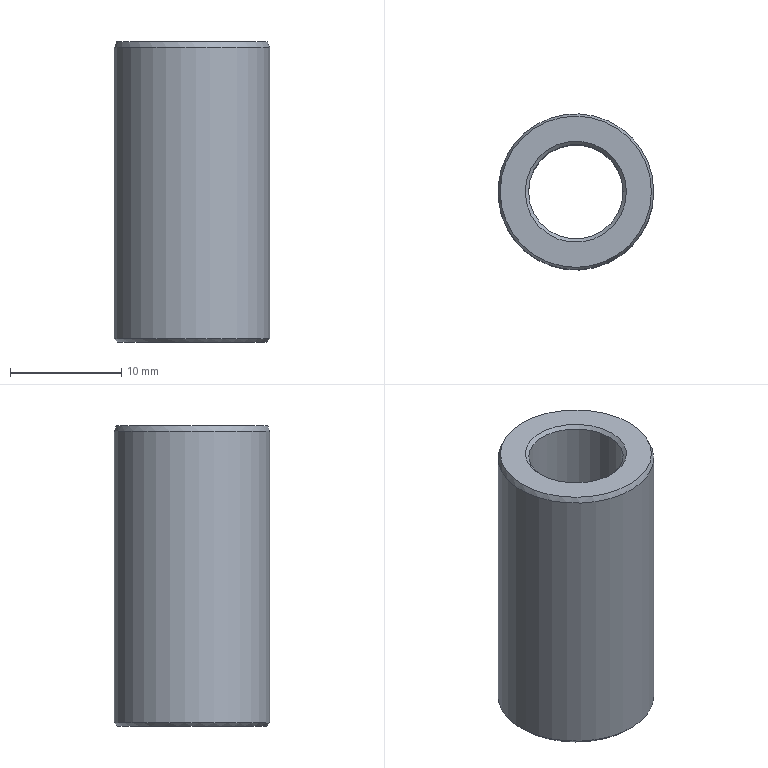Part | STEP file | 1 solid | 8 faces | box 14 x 14 x 27 mm | volume 2618 mm3 | cone 4 | cylinder 2 | plane 2 | commonest cylinder face diameters 8.5 x1 14 x1
STEP:
#1=CARTESIAN_POINT('',(0.,0.,0.));
#2=DIRECTION('',(0.,0.,1.));
#3=DIRECTION('',(1.,0.,0.));
#4=AXIS2_PLACEMENT_3D('',#1,#2,#3);
#5=CARTESIAN_POINT('',(1324.247,352.48,-53.881));
#6=VERTEX_POINT('',#5);
#7=CARTESIAN_POINT('',(1317.247,352.48,-53.881));
#8=DIRECTION('',(0.,0.,-1.));
#9=DIRECTION('',(1.,0.,0.));
#10=AXIS2_PLACEMENT_3D('',#7,#8,#9);
#11=CIRCLE('',#10,7.);
#12=CARTESIAN_POINT('',(1317.247,352.48,-53.381));
#13=DIRECTION('',(0.,0.,-1.));
#14=DIRECTION('',(-1.,0.,0.));
#15=AXIS2_PLACEMENT_3D('',#12,#13,#14);
#16=CYLINDRICAL_SURFACE('',#15,7.);
#17=CARTESIAN_POINT('',(3.142,0.5));
#18=DIRECTION('',(1.,0.));
#19=VECTOR('',#18,1.);
#20=LINE('',#17,#19);
#21=(GEOMETRIC_REPRESENTATION_CONTEXT(2)PARAMETRIC_REPRESENTATION_CONTEXT()REPRESENTATION_CONTEXT('',''));
#22=DEFINITIONAL_REPRESENTATION('',(#20),#21);
#23=PCURVE('',#16,#22);
#24=CARTESIAN_POINT('',(1317.247,352.48,-53.881));
#25=DIRECTION('',(0.,0.,-1.));
#26=DIRECTION('',(-1.,0.,0.));
#27=AXIS2_PLACEMENT_3D('',#24,#25,#26);
#28=CONICAL_SURFACE('',#27,7.,0.3927);
#29=CARTESIAN_POINT('',(3.142,0.));
#30=DIRECTION('',(1.,0.));
#31=VECTOR('',#30,1.);
#32=LINE('',#29,#31);
#33=(GEOMETRIC_REPRESENTATION_CONTEXT(2)PARAMETRIC_REPRESENTATION_CONTEXT()REPRESENTATION_CONTEXT('',''));
#34=DEFINITIONAL_REPRESENTATION('',(#32),#33);
#35=PCURVE('',#28,#34);
#36=SURFACE_CURVE('',#11,(#23,#35),.PCURVE_S1.);
#37=EDGE_CURVE('',#6,#6,#36,.T.);
#38=ORIENTED_EDGE('',*,*,#37,.T.);
#39=CARTESIAN_POINT('',(1324.247,352.48,-80.081));
#40=VERTEX_POINT('',#39);
#41=CARTESIAN_POINT('',(1324.247,352.48,-53.881));
#42=CARTESIAN_POINT('',(1324.247,352.48,-80.081));
#43=B_SPLINE_CURVE_WITH_KNOTS('',1,(#41,#42),.UNSPECIFIED.,.F.,.F.,(2,2),(0.5,26.7),.PIECEWISE_BEZIER_KNOTS.);
#44=CARTESIAN_POINT('',(9.425,0.));
#45=DIRECTION('',(0.,1.));
#46=VECTOR('',#45,1.);
#47=LINE('',#44,#46);
#48=(GEOMETRIC_REPRESENTATION_CONTEXT(2)PARAMETRIC_REPRESENTATION_CONTEXT()REPRESENTATION_CONTEXT('',''));
#49=DEFINITIONAL_REPRESENTATION('',(#47),#48);
#50=PCURVE('',#16,#49);
#51=CARTESIAN_POINT('',(3.142,0.));
#52=DIRECTION('',(0.,1.));
#53=VECTOR('',#52,1.);
#54=LINE('',#51,#53);
#55=(GEOMETRIC_REPRESENTATION_CONTEXT(2)PARAMETRIC_REPRESENTATION_CONTEXT()REPRESENTATION_CONTEXT('',''));
#56=DEFINITIONAL_REPRESENTATION('',(#54),#55);
#57=PCURVE('',#16,#56);
#58=SEAM_CURVE('',#43,(#50,#57),.PCURVE_S1.);
#59=EDGE_CURVE('',#6,#40,#58,.T.);
#60=ORIENTED_EDGE('',*,*,#59,.T.);
#61=CARTESIAN_POINT('',(1317.247,352.48,-80.081));
#62=DIRECTION('',(0.,0.,1.));
#63=DIRECTION('',(1.,0.,0.));
#64=AXIS2_PLACEMENT_3D('',#61,#62,#63);
#65=CIRCLE('',#64,7.);
#66=CARTESIAN_POINT('',(9.425,26.7));
#67=DIRECTION('',(-1.,0.));
#68=VECTOR('',#67,1.);
#69=LINE('',#66,#68);
#70=(GEOMETRIC_REPRESENTATION_CONTEXT(2)PARAMETRIC_REPRESENTATION_CONTEXT()REPRESENTATION_CONTEXT('',''));
#71=DEFINITIONAL_REPRESENTATION('',(#69),#70);
#72=PCURVE('',#16,#71);
#73=CARTESIAN_POINT('',(1317.247,352.48,-80.381));
#74=DIRECTION('',(0.,0.,1.));
#75=DIRECTION('',(1.,0.,0.));
#76=AXIS2_PLACEMENT_3D('',#73,#74,#75);
#77=CONICAL_SURFACE('',#76,6.7,0.7854);
#78=CARTESIAN_POINT('',(0.,0.3));
#79=DIRECTION('',(1.,0.));
#80=VECTOR('',#79,1.);
#81=LINE('',#78,#80);
#82=(GEOMETRIC_REPRESENTATION_CONTEXT(2)PARAMETRIC_REPRESENTATION_CONTEXT()REPRESENTATION_CONTEXT('',''));
#83=DEFINITIONAL_REPRESENTATION('',(#81),#82);
#84=PCURVE('',#77,#83);
#85=SURFACE_CURVE('',#65,(#72,#84),.PCURVE_S1.);
#86=EDGE_CURVE('',#40,#40,#85,.T.);
#87=ORIENTED_EDGE('',*,*,#86,.T.);
#88=ORIENTED_EDGE('',*,*,#59,.F.);
#89=EDGE_LOOP('',(#38,#60,#87,#88));
#90=FACE_BOUND('',#89,.T.);
#91=ADVANCED_FACE('',(#90),#16,.T.);
#92=CARTESIAN_POINT('',(1321.797,352.48,-53.381));
#93=VERTEX_POINT('',#92);
#94=CARTESIAN_POINT('',(1317.247,352.48,-53.381));
#95=DIRECTION('',(0.,0.,-1.));
#96=DIRECTION('',(1.,0.,0.));
#97=AXIS2_PLACEMENT_3D('',#94,#95,#96);
#98=CIRCLE('',#97,4.55);
#99=CARTESIAN_POINT('',(1317.247,352.48,-53.381));
#100=DIRECTION('',(0.,0.,1.));
#101=DIRECTION('',(-1.,0.,0.));
#102=AXIS2_PLACEMENT_3D('',#99,#100,#101);
#103=PLANE('',#102);
#104=CARTESIAN_POINT('',(-4.55,0.));
#105=CARTESIAN_POINT('',(-4.55,7.881));
#106=CARTESIAN_POINT('',(2.275,3.94));
#107=CARTESIAN_POINT('',(9.1,0.));
#108=CARTESIAN_POINT('',(2.275,-3.94));
#109=CARTESIAN_POINT('',(-4.55,-7.881));
#110=CARTESIAN_POINT('',(-4.55,0.));
#111=(BOUNDED_CURVE()B_SPLINE_CURVE(2,(#104,#105,#106,#107,#108,#109,#110),.UNSPECIFIED.,.T.,.F.)B_SPLINE_CURVE_WITH_KNOTS((1,2,2,2,2,1),(-2.094,0.,2.094,4.189,6.283,8.378),.UNSPECIFIED.)CURVE()GEOMETRIC_REPRESENTATION_ITEM()RATIONAL_B_SPLINE_CURVE((1.,0.5,1.,0.5,1.,0.5,1.))REPRESENTATION_ITEM(''));
#112=(GEOMETRIC_REPRESENTATION_CONTEXT(2)PARAMETRIC_REPRESENTATION_CONTEXT()REPRESENTATION_CONTEXT('',''));
#113=DEFINITIONAL_REPRESENTATION('',(#111),#112);
#114=PCURVE('',#103,#113);
#115=CARTESIAN_POINT('',(1317.247,352.48,-53.681));
#116=DIRECTION('',(0.,0.,1.));
#117=DIRECTION('',(1.,0.,0.));
#118=AXIS2_PLACEMENT_3D('',#115,#116,#117);
#119=CONICAL_SURFACE('',#118,4.25,0.7854);
#120=CARTESIAN_POINT('',(6.283,0.3));
#121=DIRECTION('',(-1.,0.));
#122=VECTOR('',#121,1.);
#123=LINE('',#120,#122);
#124=(GEOMETRIC_REPRESENTATION_CONTEXT(2)PARAMETRIC_REPRESENTATION_CONTEXT()REPRESENTATION_CONTEXT('',''));
#125=DEFINITIONAL_REPRESENTATION('',(#123),#124);
#126=PCURVE('',#119,#125);
#127=SURFACE_CURVE('',#98,(#114,#126),.PCURVE_S1.);
#128=EDGE_CURVE('',#93,#93,#127,.T.);
#129=ORIENTED_EDGE('',*,*,#128,.T.);
#130=EDGE_LOOP('',(#129));
#131=FACE_BOUND('',#130,.T.);
#132=CARTESIAN_POINT('',(1324.04,352.48,-53.381));
#133=VERTEX_POINT('',#132);
#134=CARTESIAN_POINT('',(1317.247,352.48,-53.381));
#135=DIRECTION('',(0.,0.,1.));
#136=DIRECTION('',(1.,0.,0.));
#137=AXIS2_PLACEMENT_3D('',#134,#135,#136);
#138=CIRCLE('',#137,6.793);
#139=CARTESIAN_POINT('',(0.,0.));
#140=DIRECTION('',(-1.,0.));
#141=AXIS2_PLACEMENT_2D('',#139,#140);
#142=CIRCLE('',#141,6.793);
#143=(GEOMETRIC_REPRESENTATION_CONTEXT(2)PARAMETRIC_REPRESENTATION_CONTEXT()REPRESENTATION_CONTEXT('',''));
#144=DEFINITIONAL_REPRESENTATION('',(#142),#143);
#145=PCURVE('',#103,#144);
#146=CARTESIAN_POINT('',(9.425,-0.5));
#147=DIRECTION('',(-1.,0.));
#148=VECTOR('',#147,1.);
#149=LINE('',#146,#148);
#150=(GEOMETRIC_REPRESENTATION_CONTEXT(2)PARAMETRIC_REPRESENTATION_CONTEXT()REPRESENTATION_CONTEXT('',''));
#151=DEFINITIONAL_REPRESENTATION('',(#149),#150);
#152=PCURVE('',#28,#151);
#153=SURFACE_CURVE('',#138,(#145,#152),.PCURVE_S1.);
#154=EDGE_CURVE('',#133,#133,#153,.T.);
#155=ORIENTED_EDGE('',*,*,#154,.T.);
#156=EDGE_LOOP('',(#155));
#157=FACE_BOUND('',#156,.T.);
#158=ADVANCED_FACE('',(#131,#157),#103,.T.);
#159=CARTESIAN_POINT('',(1321.497,352.48,-53.681));
#160=VERTEX_POINT('',#159);
#161=CARTESIAN_POINT('',(1317.247,352.48,-53.681));
#162=DIRECTION('',(0.,0.,1.));
#163=DIRECTION('',(1.,0.,0.));
#164=AXIS2_PLACEMENT_3D('',#161,#162,#163);
#165=CIRCLE('',#164,4.25);
#166=CARTESIAN_POINT('',(1317.247,352.48,-89.381));
#167=DIRECTION('',(0.,0.,1.));
#168=DIRECTION('',(-1.,0.,0.));
#169=AXIS2_PLACEMENT_3D('',#166,#167,#168);
#170=CYLINDRICAL_SURFACE('',#169,4.25);
#171=CARTESIAN_POINT('',(3.142,35.7));
#172=DIRECTION('',(1.,0.));
#173=VECTOR('',#172,1.);
#174=LINE('',#171,#173);
#175=(GEOMETRIC_REPRESENTATION_CONTEXT(2)PARAMETRIC_REPRESENTATION_CONTEXT()REPRESENTATION_CONTEXT('',''));
#176=DEFINITIONAL_REPRESENTATION('',(#174),#175);
#177=PCURVE('',#170,#176);
#178=CARTESIAN_POINT('',(0.,0.));
#179=DIRECTION('',(1.,0.));
#180=VECTOR('',#179,1.);
#181=LINE('',#178,#180);
#182=(GEOMETRIC_REPRESENTATION_CONTEXT(2)PARAMETRIC_REPRESENTATION_CONTEXT()REPRESENTATION_CONTEXT('',''));
#183=DEFINITIONAL_REPRESENTATION('',(#181),#182);
#184=PCURVE('',#119,#183);
#185=SURFACE_CURVE('',#165,(#177,#184),.PCURVE_S1.);
#186=EDGE_CURVE('',#160,#160,#185,.T.);
#187=ORIENTED_EDGE('',*,*,#186,.F.);
#188=CARTESIAN_POINT('',(1321.497,352.48,-80.081));
#189=VERTEX_POINT('',#188);
#190=CARTESIAN_POINT('',(1321.497,352.48,-80.081));
#191=CARTESIAN_POINT('',(1321.497,352.48,-53.681));
#192=B_SPLINE_CURVE_WITH_KNOTS('',1,(#190,#191),.UNSPECIFIED.,.F.,.F.,(2,2),(9.3,35.7),.PIECEWISE_BEZIER_KNOTS.);
#193=CARTESIAN_POINT('',(3.142,0.));
#194=DIRECTION('',(0.,1.));
#195=VECTOR('',#194,1.);
#196=LINE('',#193,#195);
#197=(GEOMETRIC_REPRESENTATION_CONTEXT(2)PARAMETRIC_REPRESENTATION_CONTEXT()REPRESENTATION_CONTEXT('',''));
#198=DEFINITIONAL_REPRESENTATION('',(#196),#197);
#199=PCURVE('',#170,#198);
#200=CARTESIAN_POINT('',(9.425,0.));
#201=DIRECTION('',(0.,1.));
#202=VECTOR('',#201,1.);
#203=LINE('',#200,#202);
#204=(GEOMETRIC_REPRESENTATION_CONTEXT(2)PARAMETRIC_REPRESENTATION_CONTEXT()REPRESENTATION_CONTEXT('',''));
#205=DEFINITIONAL_REPRESENTATION('',(#203),#204);
#206=PCURVE('',#170,#205);
#207=SEAM_CURVE('',#192,(#199,#206),.PCURVE_S1.);
#208=EDGE_CURVE('',#189,#160,#207,.T.);
#209=ORIENTED_EDGE('',*,*,#208,.F.);
#210=CARTESIAN_POINT('',(1317.247,352.48,-80.081));
#211=DIRECTION('',(0.,0.,-1.));
#212=DIRECTION('',(1.,0.,0.));
#213=AXIS2_PLACEMENT_3D('',#210,#211,#212);
#214=CIRCLE('',#213,4.25);
#215=CARTESIAN_POINT('',(9.425,9.3));
#216=DIRECTION('',(-1.,0.));
#217=VECTOR('',#216,1.);
#218=LINE('',#215,#217);
#219=(GEOMETRIC_REPRESENTATION_CONTEXT(2)PARAMETRIC_REPRESENTATION_CONTEXT()REPRESENTATION_CONTEXT('',''));
#220=DEFINITIONAL_REPRESENTATION('',(#218),#219);
#221=PCURVE('',#170,#220);
#222=CARTESIAN_POINT('',(1317.247,352.48,-80.081));
#223=DIRECTION('',(0.,0.,-1.));
#224=DIRECTION('',(-1.,0.,0.));
#225=AXIS2_PLACEMENT_3D('',#222,#223,#224);
#226=CONICAL_SURFACE('',#225,4.25,0.7854);
#227=CARTESIAN_POINT('',(3.142,0.));
#228=DIRECTION('',(1.,0.));
#229=VECTOR('',#228,1.);
#230=LINE('',#227,#229);
#231=(GEOMETRIC_REPRESENTATION_CONTEXT(2)PARAMETRIC_REPRESENTATION_CONTEXT()REPRESENTATION_CONTEXT('',''));
#232=DEFINITIONAL_REPRESENTATION('',(#230),#231);
#233=PCURVE('',#226,#232);
#234=SURFACE_CURVE('',#214,(#221,#233),.PCURVE_S1.);
#235=EDGE_CURVE('',#189,#189,#234,.T.);
#236=ORIENTED_EDGE('',*,*,#235,.F.);
#237=ORIENTED_EDGE('',*,*,#208,.T.);
#238=EDGE_LOOP('',(#187,#209,#236,#237));
#239=FACE_BOUND('',#238,.F.);
#240=ADVANCED_FACE('',(#239),#170,.F.);
#241=CARTESIAN_POINT('',(1323.947,352.48,-80.381));
#242=VERTEX_POINT('',#241);
#243=CARTESIAN_POINT('',(1317.247,352.48,-80.381));
#244=DIRECTION('',(0.,0.,-1.));
#245=DIRECTION('',(1.,0.,0.));
#246=AXIS2_PLACEMENT_3D('',#243,#244,#245);
#247=CIRCLE('',#246,6.7);
#248=CARTESIAN_POINT('',(1317.247,352.48,-80.381));
#249=DIRECTION('',(0.,0.,1.));
#250=DIRECTION('',(1.,0.,0.));
#251=AXIS2_PLACEMENT_3D('',#248,#249,#250);
#252=PLANE('',#251);
#253=CARTESIAN_POINT('',(6.7,0.));
#254=CARTESIAN_POINT('',(6.7,-11.605));
#255=CARTESIAN_POINT('',(-3.35,-5.802));
#256=CARTESIAN_POINT('',(-13.4,0.));
#257=CARTESIAN_POINT('',(-3.35,5.802));
#258=CARTESIAN_POINT('',(6.7,11.605));
#259=CARTESIAN_POINT('',(6.7,0.));
#260=(BOUNDED_CURVE()B_SPLINE_CURVE(2,(#253,#254,#255,#256,#257,#258,#259),.UNSPECIFIED.,.T.,.F.)B_SPLINE_CURVE_WITH_KNOTS((1,2,2,2,2,1),(-2.094,0.,2.094,4.189,6.283,8.378),.UNSPECIFIED.)CURVE()GEOMETRIC_REPRESENTATION_ITEM()RATIONAL_B_SPLINE_CURVE((1.,0.5,1.,0.5,1.,0.5,1.))REPRESENTATION_ITEM(''));
#261=(GEOMETRIC_REPRESENTATION_CONTEXT(2)PARAMETRIC_REPRESENTATION_CONTEXT()REPRESENTATION_CONTEXT('',''));
#262=DEFINITIONAL_REPRESENTATION('',(#260),#261);
#263=PCURVE('',#252,#262);
#264=CARTESIAN_POINT('',(6.283,0.));
#265=DIRECTION('',(-1.,0.));
#266=VECTOR('',#265,1.);
#267=LINE('',#264,#266);
#268=(GEOMETRIC_REPRESENTATION_CONTEXT(2)PARAMETRIC_REPRESENTATION_CONTEXT()REPRESENTATION_CONTEXT('',''));
#269=DEFINITIONAL_REPRESENTATION('',(#267),#268);
#270=PCURVE('',#77,#269);
#271=SURFACE_CURVE('',#247,(#263,#270),.PCURVE_S1.);
#272=EDGE_CURVE('',#242,#242,#271,.T.);
#273=ORIENTED_EDGE('',*,*,#272,.T.);
#274=EDGE_LOOP('',(#273));
#275=FACE_BOUND('',#274,.T.);
#276=CARTESIAN_POINT('',(1321.797,352.48,-80.381));
#277=VERTEX_POINT('',#276);
#278=CARTESIAN_POINT('',(1317.247,352.48,-80.381));
#279=DIRECTION('',(0.,0.,1.));
#280=DIRECTION('',(1.,0.,0.));
#281=AXIS2_PLACEMENT_3D('',#278,#279,#280);
#282=CIRCLE('',#281,4.55);
#283=CARTESIAN_POINT('',(0.,0.));
#284=DIRECTION('',(1.,0.));
#285=AXIS2_PLACEMENT_2D('',#283,#284);
#286=CIRCLE('',#285,4.55);
#287=(GEOMETRIC_REPRESENTATION_CONTEXT(2)PARAMETRIC_REPRESENTATION_CONTEXT()REPRESENTATION_CONTEXT('',''));
#288=DEFINITIONAL_REPRESENTATION('',(#286),#287);
#289=PCURVE('',#252,#288);
#290=CARTESIAN_POINT('',(9.425,0.3));
#291=DIRECTION('',(-1.,0.));
#292=VECTOR('',#291,1.);
#293=LINE('',#290,#292);
#294=(GEOMETRIC_REPRESENTATION_CONTEXT(2)PARAMETRIC_REPRESENTATION_CONTEXT()REPRESENTATION_CONTEXT('',''));
#295=DEFINITIONAL_REPRESENTATION('',(#293),#294);
#296=PCURVE('',#226,#295);
#297=SURFACE_CURVE('',#282,(#289,#296),.PCURVE_S1.);
#298=EDGE_CURVE('',#277,#277,#297,.T.);
#299=ORIENTED_EDGE('',*,*,#298,.T.);
#300=EDGE_LOOP('',(#299));
#301=FACE_BOUND('',#300,.T.);
#302=ADVANCED_FACE('',(#275,#301),#252,.F.);
#303=ORIENTED_EDGE('',*,*,#154,.F.);
#304=CARTESIAN_POINT('',(1324.04,352.48,-53.381));
#305=CARTESIAN_POINT('',(1324.247,352.48,-53.881));
#306=B_SPLINE_CURVE_WITH_KNOTS('',1,(#304,#305),.UNSPECIFIED.,.F.,.F.,(2,2),(-0.5412,0.),.PIECEWISE_BEZIER_KNOTS.);
#307=CARTESIAN_POINT('',(9.425,0.));
#308=DIRECTION('',(0.,1.));
#309=VECTOR('',#308,1.);
#310=LINE('',#307,#309);
#311=(GEOMETRIC_REPRESENTATION_CONTEXT(2)PARAMETRIC_REPRESENTATION_CONTEXT()REPRESENTATION_CONTEXT('',''));
#312=DEFINITIONAL_REPRESENTATION('',(#310),#311);
#313=PCURVE('',#28,#312);
#314=CARTESIAN_POINT('',(3.142,0.));
#315=DIRECTION('',(0.,1.));
#316=VECTOR('',#315,1.);
#317=LINE('',#314,#316);
#318=(GEOMETRIC_REPRESENTATION_CONTEXT(2)PARAMETRIC_REPRESENTATION_CONTEXT()REPRESENTATION_CONTEXT('',''));
#319=DEFINITIONAL_REPRESENTATION('',(#317),#318);
#320=PCURVE('',#28,#319);
#321=SEAM_CURVE('',#306,(#313,#320),.PCURVE_S1.);
#322=EDGE_CURVE('',#133,#6,#321,.T.);
#323=ORIENTED_EDGE('',*,*,#322,.T.);
#324=ORIENTED_EDGE('',*,*,#37,.F.);
#325=ORIENTED_EDGE('',*,*,#322,.F.);
#326=EDGE_LOOP('',(#303,#323,#324,#325));
#327=FACE_BOUND('',#326,.T.);
#328=ADVANCED_FACE('',(#327),#28,.T.);
#329=ORIENTED_EDGE('',*,*,#86,.F.);
#330=CARTESIAN_POINT('',(1323.947,352.48,-80.381));
#331=CARTESIAN_POINT('',(1324.247,352.48,-80.081));
#332=B_SPLINE_CURVE_WITH_KNOTS('',1,(#330,#331),.UNSPECIFIED.,.F.,.F.,(2,2),(0.,0.4243),.PIECEWISE_BEZIER_KNOTS.);
#333=CARTESIAN_POINT('',(0.,0.));
#334=DIRECTION('',(0.,1.));
#335=VECTOR('',#334,1.);
#336=LINE('',#333,#335);
#337=(GEOMETRIC_REPRESENTATION_CONTEXT(2)PARAMETRIC_REPRESENTATION_CONTEXT()REPRESENTATION_CONTEXT('',''));
#338=DEFINITIONAL_REPRESENTATION('',(#336),#337);
#339=PCURVE('',#77,#338);
#340=CARTESIAN_POINT('',(6.283,0.));
#341=DIRECTION('',(0.,1.));
#342=VECTOR('',#341,1.);
#343=LINE('',#340,#342);
#344=(GEOMETRIC_REPRESENTATION_CONTEXT(2)PARAMETRIC_REPRESENTATION_CONTEXT()REPRESENTATION_CONTEXT('',''));
#345=DEFINITIONAL_REPRESENTATION('',(#343),#344);
#346=PCURVE('',#77,#345);
#347=SEAM_CURVE('',#332,(#339,#346),.PCURVE_S1.);
#348=EDGE_CURVE('',#242,#40,#347,.T.);
#349=ORIENTED_EDGE('',*,*,#348,.F.);
#350=ORIENTED_EDGE('',*,*,#272,.F.);
#351=ORIENTED_EDGE('',*,*,#348,.T.);
#352=EDGE_LOOP('',(#329,#349,#350,#351));
#353=FACE_BOUND('',#352,.T.);
#354=ADVANCED_FACE('',(#353),#77,.T.);
#355=ORIENTED_EDGE('',*,*,#298,.T.);
#356=CARTESIAN_POINT('',(1321.497,352.48,-80.081));
#357=CARTESIAN_POINT('',(1321.797,352.48,-80.381));
#358=B_SPLINE_CURVE_WITH_KNOTS('',1,(#356,#357),.UNSPECIFIED.,.F.,.F.,(2,2),(0.,0.4243),.PIECEWISE_BEZIER_KNOTS.);
#359=CARTESIAN_POINT('',(3.142,0.));
#360=DIRECTION('',(0.,1.));
#361=VECTOR('',#360,1.);
#362=LINE('',#359,#361);
#363=(GEOMETRIC_REPRESENTATION_CONTEXT(2)PARAMETRIC_REPRESENTATION_CONTEXT()REPRESENTATION_CONTEXT('',''));
#364=DEFINITIONAL_REPRESENTATION('',(#362),#363);
#365=PCURVE('',#226,#364);
#366=CARTESIAN_POINT('',(9.425,0.));
#367=DIRECTION('',(0.,1.));
#368=VECTOR('',#367,1.);
#369=LINE('',#366,#368);
#370=(GEOMETRIC_REPRESENTATION_CONTEXT(2)PARAMETRIC_REPRESENTATION_CONTEXT()REPRESENTATION_CONTEXT('',''));
#371=DEFINITIONAL_REPRESENTATION('',(#369),#370);
#372=PCURVE('',#226,#371);
#373=SEAM_CURVE('',#358,(#365,#372),.PCURVE_S1.);
#374=EDGE_CURVE('',#189,#277,#373,.T.);
#375=ORIENTED_EDGE('',*,*,#374,.F.);
#376=ORIENTED_EDGE('',*,*,#235,.T.);
#377=ORIENTED_EDGE('',*,*,#374,.T.);
#378=EDGE_LOOP('',(#355,#375,#376,#377));
#379=FACE_BOUND('',#378,.F.);
#380=ADVANCED_FACE('',(#379),#226,.F.);
#381=ORIENTED_EDGE('',*,*,#128,.T.);
#382=CARTESIAN_POINT('',(1321.497,352.48,-53.681));
#383=CARTESIAN_POINT('',(1321.797,352.48,-53.381));
#384=B_SPLINE_CURVE_WITH_KNOTS('',1,(#382,#383),.UNSPECIFIED.,.F.,.F.,(2,2),(0.,0.4243),.PIECEWISE_BEZIER_KNOTS.);
#385=CARTESIAN_POINT('',(0.,0.));
#386=DIRECTION('',(0.,1.));
#387=VECTOR('',#386,1.);
#388=LINE('',#385,#387);
#389=(GEOMETRIC_REPRESENTATION_CONTEXT(2)PARAMETRIC_REPRESENTATION_CONTEXT()REPRESENTATION_CONTEXT('',''));
#390=DEFINITIONAL_REPRESENTATION('',(#388),#389);
#391=PCURVE('',#119,#390);
#392=CARTESIAN_POINT('',(6.283,0.));
#393=DIRECTION('',(0.,1.));
#394=VECTOR('',#393,1.);
#395=LINE('',#392,#394);
#396=(GEOMETRIC_REPRESENTATION_CONTEXT(2)PARAMETRIC_REPRESENTATION_CONTEXT()REPRESENTATION_CONTEXT('',''));
#397=DEFINITIONAL_REPRESENTATION('',(#395),#396);
#398=PCURVE('',#119,#397);
#399=SEAM_CURVE('',#384,(#391,#398),.PCURVE_S1.);
#400=EDGE_CURVE('',#160,#93,#399,.T.);
#401=ORIENTED_EDGE('',*,*,#400,.F.);
#402=ORIENTED_EDGE('',*,*,#186,.T.);
#403=ORIENTED_EDGE('',*,*,#400,.T.);
#404=EDGE_LOOP('',(#381,#401,#402,#403));
#405=FACE_BOUND('',#404,.F.);
#406=ADVANCED_FACE('',(#405),#119,.F.);
#407=CLOSED_SHELL('',(#91,#158,#240,#302,#328,#354,#380,#406));
#408=MANIFOLD_SOLID_BREP('',#407);
#409=(LENGTH_UNIT()NAMED_UNIT(*)SI_UNIT(.MILLI.,.METRE.));
#410=UNCERTAINTY_MEASURE_WITH_UNIT(LENGTH_MEASURE(0.00001),#409,'','');
#411=(NAMED_UNIT(*)PLANE_ANGLE_UNIT()SI_UNIT($,.RADIAN.));
#412=(NAMED_UNIT(*)SI_UNIT($,.STERADIAN.)SOLID_ANGLE_UNIT());
#413=(GEOMETRIC_REPRESENTATION_CONTEXT(3)GLOBAL_UNCERTAINTY_ASSIGNED_CONTEXT((#410))GLOBAL_UNIT_ASSIGNED_CONTEXT((#409,#411,#412))REPRESENTATION_CONTEXT('',''));
#414=ADVANCED_BREP_SHAPE_REPRESENTATION('',(#4,#408),#413);